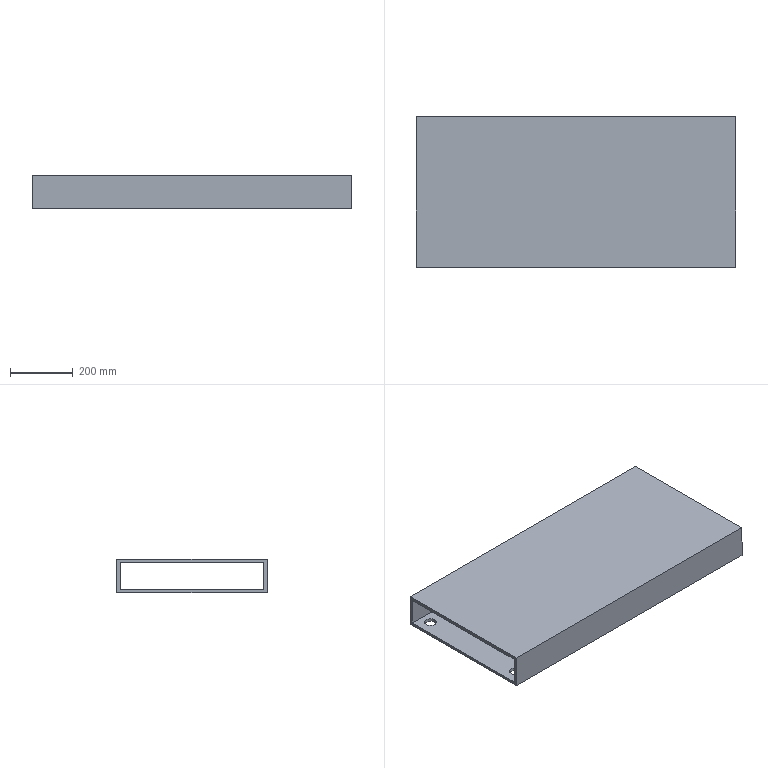Part | SolidWorks | features Cut 1, Extrusion 1, Shell 1 | 1 solid | 18 faces | box 1020 x 480 x 108 mm | volume 11543021 mm3 | plane 10 | cylinder 8 | commonest cylinder face diameters 37.5 x8
STEP:
#1=CARTESIAN_POINT('',(-446.342,191.837,10.));
#2=VERTEX_POINT('',#1);
#3=CARTESIAN_POINT('',(-483.842,191.837,10.));
#4=VERTEX_POINT('',#3);
#5=CARTESIAN_POINT('',(-465.092,191.837,10.));
#6=DIRECTION('',(0.,0.,-1.));
#7=DIRECTION('',(-1.,0.,0.));
#8=AXIS2_PLACEMENT_3D('',#5,#6,#7);
#9=CIRCLE('',#8,18.75);
#10=EDGE_CURVE('',#2,#4,#9,.T.);
#11=ORIENTED_EDGE('',*,*,#10,.F.);
#12=CARTESIAN_POINT('',(-446.342,191.837,0.));
#13=VERTEX_POINT('',#12);
#14=CARTESIAN_POINT('',(-446.342,191.837,10.));
#15=DIRECTION('',(0.,0.,-1.));
#16=VECTOR('',#15,1000.);
#17=LINE('',#14,#16);
#18=EDGE_CURVE('',#2,#13,#17,.T.);
#19=ORIENTED_EDGE('',*,*,#18,.T.);
#20=CARTESIAN_POINT('',(-483.842,191.837,0.));
#21=VERTEX_POINT('',#20);
#22=CARTESIAN_POINT('',(-465.092,191.837,0.));
#23=DIRECTION('',(0.,0.,-1.));
#24=DIRECTION('',(-1.,0.,0.));
#25=AXIS2_PLACEMENT_3D('',#22,#23,#24);
#26=CIRCLE('',#25,18.75);
#27=EDGE_CURVE('',#13,#21,#26,.T.);
#28=ORIENTED_EDGE('',*,*,#27,.T.);
#29=CARTESIAN_POINT('',(-483.842,191.837,10.));
#30=DIRECTION('',(0.,0.,-1.));
#31=VECTOR('',#30,1000.);
#32=LINE('',#29,#31);
#33=EDGE_CURVE('',#4,#21,#32,.T.);
#34=ORIENTED_EDGE('',*,*,#33,.F.);
#35=EDGE_LOOP('',(#11,#19,#28,#34));
#36=FACE_OUTER_BOUND('',#35,.T.);
#37=CARTESIAN_POINT('',(-465.092,191.837,10.));
#38=DIRECTION('',(0.,0.,-1.));
#39=DIRECTION('',(-1.,0.,0.));
#40=AXIS2_PLACEMENT_3D('',#37,#38,#39);
#41=CYLINDRICAL_SURFACE('',#40,18.75);
#42=ADVANCED_FACE('',(#36),#41,.F.);
#43=CARTESIAN_POINT('',(-446.342,-191.837,10.));
#44=VERTEX_POINT('',#43);
#45=CARTESIAN_POINT('',(-483.842,-191.837,10.));
#46=VERTEX_POINT('',#45);
#47=CARTESIAN_POINT('',(-465.092,-191.837,10.));
#48=DIRECTION('',(0.,0.,-1.));
#49=DIRECTION('',(-1.,0.,0.));
#50=AXIS2_PLACEMENT_3D('',#47,#48,#49);
#51=CIRCLE('',#50,18.75);
#52=EDGE_CURVE('',#44,#46,#51,.T.);
#53=ORIENTED_EDGE('',*,*,#52,.F.);
#54=CARTESIAN_POINT('',(-446.342,-191.837,0.));
#55=VERTEX_POINT('',#54);
#56=CARTESIAN_POINT('',(-446.342,-191.837,10.));
#57=DIRECTION('',(0.,0.,-1.));
#58=VECTOR('',#57,1000.);
#59=LINE('',#56,#58);
#60=EDGE_CURVE('',#44,#55,#59,.T.);
#61=ORIENTED_EDGE('',*,*,#60,.T.);
#62=CARTESIAN_POINT('',(-483.842,-191.837,0.));
#63=VERTEX_POINT('',#62);
#64=CARTESIAN_POINT('',(-465.092,-191.837,0.));
#65=DIRECTION('',(0.,0.,-1.));
#66=DIRECTION('',(-1.,0.,0.));
#67=AXIS2_PLACEMENT_3D('',#64,#65,#66);
#68=CIRCLE('',#67,18.75);
#69=EDGE_CURVE('',#55,#63,#68,.T.);
#70=ORIENTED_EDGE('',*,*,#69,.T.);
#71=CARTESIAN_POINT('',(-483.842,-191.837,10.));
#72=DIRECTION('',(0.,0.,-1.));
#73=VECTOR('',#72,1000.);
#74=LINE('',#71,#73);
#75=EDGE_CURVE('',#46,#63,#74,.T.);
#76=ORIENTED_EDGE('',*,*,#75,.F.);
#77=EDGE_LOOP('',(#53,#61,#70,#76));
#78=FACE_OUTER_BOUND('',#77,.T.);
#79=CARTESIAN_POINT('',(-465.092,-191.837,10.));
#80=DIRECTION('',(0.,0.,-1.));
#81=DIRECTION('',(-1.,0.,0.));
#82=AXIS2_PLACEMENT_3D('',#79,#80,#81);
#83=CYLINDRICAL_SURFACE('',#82,18.75);
#84=ADVANCED_FACE('',(#78),#83,.F.);
#85=CARTESIAN_POINT('',(414.283,-192.188,10.));
#86=VERTEX_POINT('',#85);
#87=CARTESIAN_POINT('',(376.783,-192.188,10.));
#88=VERTEX_POINT('',#87);
#89=CARTESIAN_POINT('',(395.533,-192.188,10.));
#90=DIRECTION('',(0.,0.,-1.));
#91=DIRECTION('',(-1.,0.,0.));
#92=AXIS2_PLACEMENT_3D('',#89,#90,#91);
#93=CIRCLE('',#92,18.75);
#94=EDGE_CURVE('',#86,#88,#93,.T.);
#95=ORIENTED_EDGE('',*,*,#94,.F.);
#96=CARTESIAN_POINT('',(414.283,-192.188,0.));
#97=VERTEX_POINT('',#96);
#98=CARTESIAN_POINT('',(414.283,-192.188,10.));
#99=DIRECTION('',(0.,0.,-1.));
#100=VECTOR('',#99,1000.);
#101=LINE('',#98,#100);
#102=EDGE_CURVE('',#86,#97,#101,.T.);
#103=ORIENTED_EDGE('',*,*,#102,.T.);
#104=CARTESIAN_POINT('',(376.783,-192.188,0.));
#105=VERTEX_POINT('',#104);
#106=CARTESIAN_POINT('',(395.533,-192.188,0.));
#107=DIRECTION('',(0.,0.,-1.));
#108=DIRECTION('',(-1.,0.,0.));
#109=AXIS2_PLACEMENT_3D('',#106,#107,#108);
#110=CIRCLE('',#109,18.75);
#111=EDGE_CURVE('',#97,#105,#110,.T.);
#112=ORIENTED_EDGE('',*,*,#111,.T.);
#113=CARTESIAN_POINT('',(376.783,-192.188,10.));
#114=DIRECTION('',(0.,0.,-1.));
#115=VECTOR('',#114,1000.);
#116=LINE('',#113,#115);
#117=EDGE_CURVE('',#88,#105,#116,.T.);
#118=ORIENTED_EDGE('',*,*,#117,.F.);
#119=EDGE_LOOP('',(#95,#103,#112,#118));
#120=FACE_OUTER_BOUND('',#119,.T.);
#121=CARTESIAN_POINT('',(395.533,-192.188,10.));
#122=DIRECTION('',(0.,0.,-1.));
#123=DIRECTION('',(-1.,0.,0.));
#124=AXIS2_PLACEMENT_3D('',#121,#122,#123);
#125=CYLINDRICAL_SURFACE('',#124,18.75);
#126=ADVANCED_FACE('',(#120),#125,.F.);
#127=CARTESIAN_POINT('',(416.221,192.187,10.));
#128=VERTEX_POINT('',#127);
#129=CARTESIAN_POINT('',(378.721,192.187,10.));
#130=VERTEX_POINT('',#129);
#131=CARTESIAN_POINT('',(397.471,192.187,10.));
#132=DIRECTION('',(0.,0.,-1.));
#133=DIRECTION('',(-1.,0.,0.));
#134=AXIS2_PLACEMENT_3D('',#131,#132,#133);
#135=CIRCLE('',#134,18.75);
#136=EDGE_CURVE('',#128,#130,#135,.T.);
#137=ORIENTED_EDGE('',*,*,#136,.F.);
#138=CARTESIAN_POINT('',(416.221,192.187,0.));
#139=VERTEX_POINT('',#138);
#140=CARTESIAN_POINT('',(416.221,192.187,10.));
#141=DIRECTION('',(0.,0.,-1.));
#142=VECTOR('',#141,1000.);
#143=LINE('',#140,#142);
#144=EDGE_CURVE('',#128,#139,#143,.T.);
#145=ORIENTED_EDGE('',*,*,#144,.T.);
#146=CARTESIAN_POINT('',(378.721,192.187,0.));
#147=VERTEX_POINT('',#146);
#148=CARTESIAN_POINT('',(397.471,192.187,0.));
#149=DIRECTION('',(0.,0.,-1.));
#150=DIRECTION('',(-1.,0.,0.));
#151=AXIS2_PLACEMENT_3D('',#148,#149,#150);
#152=CIRCLE('',#151,18.75);
#153=EDGE_CURVE('',#139,#147,#152,.T.);
#154=ORIENTED_EDGE('',*,*,#153,.T.);
#155=CARTESIAN_POINT('',(378.721,192.187,10.));
#156=DIRECTION('',(0.,0.,-1.));
#157=VECTOR('',#156,1000.);
#158=LINE('',#155,#157);
#159=EDGE_CURVE('',#130,#147,#158,.T.);
#160=ORIENTED_EDGE('',*,*,#159,.F.);
#161=EDGE_LOOP('',(#137,#145,#154,#160));
#162=FACE_OUTER_BOUND('',#161,.T.);
#163=CARTESIAN_POINT('',(397.471,192.187,10.));
#164=DIRECTION('',(0.,0.,-1.));
#165=DIRECTION('',(-1.,0.,0.));
#166=AXIS2_PLACEMENT_3D('',#163,#164,#165);
#167=CYLINDRICAL_SURFACE('',#166,18.75);
#168=ADVANCED_FACE('',(#162),#167,.F.);
#169=CARTESIAN_POINT('',(510.,-240.,0.));
#170=VERTEX_POINT('',#169);
#171=CARTESIAN_POINT('',(510.,240.,0.));
#172=VERTEX_POINT('',#171);
#173=CARTESIAN_POINT('',(510.,240.,0.));
#174=DIRECTION('',(0.,1.,0.));
#175=VECTOR('',#174,1000.);
#176=LINE('',#173,#175);
#177=EDGE_CURVE('',#170,#172,#176,.T.);
#178=ORIENTED_EDGE('',*,*,#177,.T.);
#179=CARTESIAN_POINT('',(510.,240.,108.));
#180=VERTEX_POINT('',#179);
#181=CARTESIAN_POINT('',(510.,240.,108.));
#182=DIRECTION('',(0.,0.,-1.));
#183=VECTOR('',#182,1000.);
#184=LINE('',#181,#183);
#185=EDGE_CURVE('',#180,#172,#184,.T.);
#186=ORIENTED_EDGE('',*,*,#185,.F.);
#187=CARTESIAN_POINT('',(510.,-240.,108.));
#188=VERTEX_POINT('',#187);
#189=CARTESIAN_POINT('',(510.,240.,108.));
#190=DIRECTION('',(0.,1.,0.));
#191=VECTOR('',#190,1000.);
#192=LINE('',#189,#191);
#193=EDGE_CURVE('',#188,#180,#192,.T.);
#194=ORIENTED_EDGE('',*,*,#193,.F.);
#195=CARTESIAN_POINT('',(510.,-240.,108.));
#196=DIRECTION('',(0.,0.,-1.));
#197=VECTOR('',#196,1000.);
#198=LINE('',#195,#197);
#199=EDGE_CURVE('',#188,#170,#198,.T.);
#200=ORIENTED_EDGE('',*,*,#199,.T.);
#201=EDGE_LOOP('',(#178,#186,#194,#200));
#202=FACE_OUTER_BOUND('',#201,.T.);
#203=CARTESIAN_POINT('',(510.,-230.,10.));
#204=VERTEX_POINT('',#203);
#205=CARTESIAN_POINT('',(510.,230.,10.));
#206=VERTEX_POINT('',#205);
#207=CARTESIAN_POINT('',(510.,240.,10.));
#208=DIRECTION('',(0.,1.,0.));
#209=VECTOR('',#208,1000.);
#210=LINE('',#207,#209);
#211=EDGE_CURVE('',#204,#206,#210,.T.);
#212=ORIENTED_EDGE('',*,*,#211,.F.);
#213=CARTESIAN_POINT('',(510.,-230.,98.));
#214=VERTEX_POINT('',#213);
#215=CARTESIAN_POINT('',(510.,-230.,108.));
#216=DIRECTION('',(0.,0.,-1.));
#217=VECTOR('',#216,1000.);
#218=LINE('',#215,#217);
#219=EDGE_CURVE('',#214,#204,#218,.T.);
#220=ORIENTED_EDGE('',*,*,#219,.F.);
#221=CARTESIAN_POINT('',(510.,230.,98.));
#222=VERTEX_POINT('',#221);
#223=CARTESIAN_POINT('',(510.,240.,98.));
#224=DIRECTION('',(0.,1.,0.));
#225=VECTOR('',#224,1000.);
#226=LINE('',#223,#225);
#227=EDGE_CURVE('',#214,#222,#226,.T.);
#228=ORIENTED_EDGE('',*,*,#227,.T.);
#229=CARTESIAN_POINT('',(510.,230.,108.));
#230=DIRECTION('',(0.,0.,-1.));
#231=VECTOR('',#230,1000.);
#232=LINE('',#229,#231);
#233=EDGE_CURVE('',#222,#206,#232,.T.);
#234=ORIENTED_EDGE('',*,*,#233,.T.);
#235=EDGE_LOOP('',(#212,#220,#228,#234));
#236=FACE_BOUND('',#235,.T.);
#237=CARTESIAN_POINT('',(510.,240.,108.));
#238=DIRECTION('',(-1.,0.,0.));
#239=DIRECTION('',(0.,-1.,0.));
#240=AXIS2_PLACEMENT_3D('',#237,#238,#239);
#241=PLANE('',#240);
#242=ADVANCED_FACE('',(#202,#236),#241,.F.);
#243=CARTESIAN_POINT('',(-510.,240.,0.));
#244=VERTEX_POINT('',#243);
#245=CARTESIAN_POINT('',(-510.,-240.,0.));
#246=VERTEX_POINT('',#245);
#247=CARTESIAN_POINT('',(-510.,240.,0.));
#248=DIRECTION('',(0.,-1.,0.));
#249=VECTOR('',#248,1000.);
#250=LINE('',#247,#249);
#251=EDGE_CURVE('',#244,#246,#250,.T.);
#252=ORIENTED_EDGE('',*,*,#251,.T.);
#253=CARTESIAN_POINT('',(-510.,-240.,108.));
#254=VERTEX_POINT('',#253);
#255=CARTESIAN_POINT('',(-510.,-240.,108.));
#256=DIRECTION('',(0.,0.,-1.));
#257=VECTOR('',#256,1000.);
#258=LINE('',#255,#257);
#259=EDGE_CURVE('',#254,#246,#258,.T.);
#260=ORIENTED_EDGE('',*,*,#259,.F.);
#261=CARTESIAN_POINT('',(-510.,240.,108.));
#262=VERTEX_POINT('',#261);
#263=CARTESIAN_POINT('',(-510.,240.,108.));
#264=DIRECTION('',(0.,-1.,0.));
#265=VECTOR('',#264,1000.);
#266=LINE('',#263,#265);
#267=EDGE_CURVE('',#262,#254,#266,.T.);
#268=ORIENTED_EDGE('',*,*,#267,.F.);
#269=CARTESIAN_POINT('',(-510.,240.,108.));
#270=DIRECTION('',(0.,0.,-1.));
#271=VECTOR('',#270,1000.);
#272=LINE('',#269,#271);
#273=EDGE_CURVE('',#262,#244,#272,.T.);
#274=ORIENTED_EDGE('',*,*,#273,.T.);
#275=EDGE_LOOP('',(#252,#260,#268,#274));
#276=FACE_OUTER_BOUND('',#275,.T.);
#277=CARTESIAN_POINT('',(-510.,230.,10.));
#278=VERTEX_POINT('',#277);
#279=CARTESIAN_POINT('',(-510.,-230.,10.));
#280=VERTEX_POINT('',#279);
#281=CARTESIAN_POINT('',(-510.,240.,10.));
#282=DIRECTION('',(0.,-1.,0.));
#283=VECTOR('',#282,1000.);
#284=LINE('',#281,#283);
#285=EDGE_CURVE('',#278,#280,#284,.T.);
#286=ORIENTED_EDGE('',*,*,#285,.F.);
#287=CARTESIAN_POINT('',(-510.,230.,98.));
#288=VERTEX_POINT('',#287);
#289=CARTESIAN_POINT('',(-510.,230.,108.));
#290=DIRECTION('',(0.,0.,-1.));
#291=VECTOR('',#290,1000.);
#292=LINE('',#289,#291);
#293=EDGE_CURVE('',#288,#278,#292,.T.);
#294=ORIENTED_EDGE('',*,*,#293,.F.);
#295=CARTESIAN_POINT('',(-510.,-230.,98.));
#296=VERTEX_POINT('',#295);
#297=CARTESIAN_POINT('',(-510.,240.,98.));
#298=DIRECTION('',(0.,-1.,0.));
#299=VECTOR('',#298,1000.);
#300=LINE('',#297,#299);
#301=EDGE_CURVE('',#288,#296,#300,.T.);
#302=ORIENTED_EDGE('',*,*,#301,.T.);
#303=CARTESIAN_POINT('',(-510.,-230.,108.));
#304=DIRECTION('',(0.,0.,-1.));
#305=VECTOR('',#304,1000.);
#306=LINE('',#303,#305);
#307=EDGE_CURVE('',#296,#280,#306,.T.);
#308=ORIENTED_EDGE('',*,*,#307,.T.);
#309=EDGE_LOOP('',(#286,#294,#302,#308));
#310=FACE_BOUND('',#309,.T.);
#311=CARTESIAN_POINT('',(-510.,240.,108.));
#312=DIRECTION('',(1.,0.,0.));
#313=DIRECTION('',(0.,1.,0.));
#314=AXIS2_PLACEMENT_3D('',#311,#312,#313);
#315=PLANE('',#314);
#316=ADVANCED_FACE('',(#276,#310),#315,.F.);
#317=CARTESIAN_POINT('',(-510.,240.,0.));
#318=DIRECTION('',(-1.,0.,0.));
#319=VECTOR('',#318,1000.);
#320=LINE('',#317,#319);
#321=EDGE_CURVE('',#172,#244,#320,.T.);
#322=ORIENTED_EDGE('',*,*,#321,.T.);
#323=ORIENTED_EDGE('',*,*,#273,.F.);
#324=CARTESIAN_POINT('',(-510.,240.,108.));
#325=DIRECTION('',(-1.,0.,0.));
#326=VECTOR('',#325,1000.);
#327=LINE('',#324,#326);
#328=EDGE_CURVE('',#180,#262,#327,.T.);
#329=ORIENTED_EDGE('',*,*,#328,.F.);
#330=ORIENTED_EDGE('',*,*,#185,.T.);
#331=EDGE_LOOP('',(#322,#323,#329,#330));
#332=FACE_OUTER_BOUND('',#331,.T.);
#333=CARTESIAN_POINT('',(-510.,240.,108.));
#334=DIRECTION('',(0.,-1.,0.));
#335=DIRECTION('',(0.,0.,-1.));
#336=AXIS2_PLACEMENT_3D('',#333,#334,#335);
#337=PLANE('',#336);
#338=ADVANCED_FACE('',(#332),#337,.F.);
#339=CARTESIAN_POINT('',(-510.,-240.,0.));
#340=DIRECTION('',(1.,0.,0.));
#341=VECTOR('',#340,1000.);
#342=LINE('',#339,#341);
#343=EDGE_CURVE('',#246,#170,#342,.T.);
#344=ORIENTED_EDGE('',*,*,#343,.T.);
#345=ORIENTED_EDGE('',*,*,#199,.F.);
#346=CARTESIAN_POINT('',(-510.,-240.,108.));
#347=DIRECTION('',(1.,0.,0.));
#348=VECTOR('',#347,1000.);
#349=LINE('',#346,#348);
#350=EDGE_CURVE('',#254,#188,#349,.T.);
#351=ORIENTED_EDGE('',*,*,#350,.F.);
#352=ORIENTED_EDGE('',*,*,#259,.T.);
#353=EDGE_LOOP('',(#344,#345,#351,#352));
#354=FACE_OUTER_BOUND('',#353,.T.);
#355=CARTESIAN_POINT('',(-510.,-240.,108.));
#356=DIRECTION('',(0.,1.,0.));
#357=DIRECTION('',(0.,0.,1.));
#358=AXIS2_PLACEMENT_3D('',#355,#356,#357);
#359=PLANE('',#358);
#360=ADVANCED_FACE('',(#354),#359,.F.);
#361=ORIENTED_EDGE('',*,*,#193,.T.);
#362=ORIENTED_EDGE('',*,*,#328,.T.);
#363=ORIENTED_EDGE('',*,*,#267,.T.);
#364=ORIENTED_EDGE('',*,*,#350,.T.);
#365=EDGE_LOOP('',(#361,#362,#363,#364));
#366=FACE_OUTER_BOUND('',#365,.T.);
#367=CARTESIAN_POINT('',(0.,0.,108.));
#368=DIRECTION('',(0.,0.,1.));
#369=DIRECTION('',(1.,0.,0.));
#370=AXIS2_PLACEMENT_3D('',#367,#368,#369);
#371=PLANE('',#370);
#372=ADVANCED_FACE('',(#366),#371,.T.);
#373=CARTESIAN_POINT('',(-465.092,191.837,0.));
#374=DIRECTION('',(0.,0.,-1.));
#375=DIRECTION('',(-1.,0.,0.));
#376=AXIS2_PLACEMENT_3D('',#373,#374,#375);
#377=CIRCLE('',#376,18.75);
#378=EDGE_CURVE('',#21,#13,#377,.T.);
#379=ORIENTED_EDGE('',*,*,#378,.F.);
#380=ORIENTED_EDGE('',*,*,#27,.F.);
#381=EDGE_LOOP('',(#379,#380));
#382=FACE_BOUND('',#381,.T.);
#383=CARTESIAN_POINT('',(-465.092,-191.837,0.));
#384=DIRECTION('',(0.,0.,-1.));
#385=DIRECTION('',(-1.,0.,0.));
#386=AXIS2_PLACEMENT_3D('',#383,#384,#385);
#387=CIRCLE('',#386,18.75);
#388=EDGE_CURVE('',#63,#55,#387,.T.);
#389=ORIENTED_EDGE('',*,*,#388,.F.);
#390=ORIENTED_EDGE('',*,*,#69,.F.);
#391=EDGE_LOOP('',(#389,#390));
#392=FACE_BOUND('',#391,.T.);
#393=CARTESIAN_POINT('',(395.533,-192.188,0.));
#394=DIRECTION('',(0.,0.,-1.));
#395=DIRECTION('',(-1.,0.,0.));
#396=AXIS2_PLACEMENT_3D('',#393,#394,#395);
#397=CIRCLE('',#396,18.75);
#398=EDGE_CURVE('',#105,#97,#397,.T.);
#399=ORIENTED_EDGE('',*,*,#398,.F.);
#400=ORIENTED_EDGE('',*,*,#111,.F.);
#401=EDGE_LOOP('',(#399,#400));
#402=FACE_BOUND('',#401,.T.);
#403=CARTESIAN_POINT('',(397.471,192.187,0.));
#404=DIRECTION('',(0.,0.,-1.));
#405=DIRECTION('',(-1.,0.,0.));
#406=AXIS2_PLACEMENT_3D('',#403,#404,#405);
#407=CIRCLE('',#406,18.75);
#408=EDGE_CURVE('',#147,#139,#407,.T.);
#409=ORIENTED_EDGE('',*,*,#408,.F.);
#410=ORIENTED_EDGE('',*,*,#153,.F.);
#411=EDGE_LOOP('',(#409,#410));
#412=FACE_BOUND('',#411,.T.);
#413=ORIENTED_EDGE('',*,*,#177,.F.);
#414=ORIENTED_EDGE('',*,*,#343,.F.);
#415=ORIENTED_EDGE('',*,*,#251,.F.);
#416=ORIENTED_EDGE('',*,*,#321,.F.);
#417=EDGE_LOOP('',(#413,#414,#415,#416));
#418=FACE_OUTER_BOUND('',#417,.T.);
#419=CARTESIAN_POINT('',(0.,0.,0.));
#420=DIRECTION('',(0.,0.,1.));
#421=DIRECTION('',(1.,0.,0.));
#422=AXIS2_PLACEMENT_3D('',#419,#420,#421);
#423=PLANE('',#422);
#424=ADVANCED_FACE('',(#382,#392,#402,#412,#418),#423,.F.);
#425=CARTESIAN_POINT('',(-510.,230.,10.));
#426=DIRECTION('',(-1.,0.,0.));
#427=VECTOR('',#426,1000.);
#428=LINE('',#425,#427);
#429=EDGE_CURVE('',#206,#278,#428,.T.);
#430=ORIENTED_EDGE('',*,*,#429,.F.);
#431=ORIENTED_EDGE('',*,*,#233,.F.);
#432=CARTESIAN_POINT('',(-510.,230.,98.));
#433=DIRECTION('',(-1.,0.,0.));
#434=VECTOR('',#433,1000.);
#435=LINE('',#432,#434);
#436=EDGE_CURVE('',#222,#288,#435,.T.);
#437=ORIENTED_EDGE('',*,*,#436,.T.);
#438=ORIENTED_EDGE('',*,*,#293,.T.);
#439=EDGE_LOOP('',(#430,#431,#437,#438));
#440=FACE_OUTER_BOUND('',#439,.T.);
#441=CARTESIAN_POINT('',(-510.,230.,108.));
#442=DIRECTION('',(0.,-1.,0.));
#443=DIRECTION('',(0.,0.,-1.));
#444=AXIS2_PLACEMENT_3D('',#441,#442,#443);
#445=PLANE('',#444);
#446=ADVANCED_FACE('',(#440),#445,.T.);
#447=CARTESIAN_POINT('',(-510.,-230.,10.));
#448=DIRECTION('',(1.,0.,0.));
#449=VECTOR('',#448,1000.);
#450=LINE('',#447,#449);
#451=EDGE_CURVE('',#280,#204,#450,.T.);
#452=ORIENTED_EDGE('',*,*,#451,.F.);
#453=ORIENTED_EDGE('',*,*,#307,.F.);
#454=CARTESIAN_POINT('',(-510.,-230.,98.));
#455=DIRECTION('',(1.,0.,0.));
#456=VECTOR('',#455,1000.);
#457=LINE('',#454,#456);
#458=EDGE_CURVE('',#296,#214,#457,.T.);
#459=ORIENTED_EDGE('',*,*,#458,.T.);
#460=ORIENTED_EDGE('',*,*,#219,.T.);
#461=EDGE_LOOP('',(#452,#453,#459,#460));
#462=FACE_OUTER_BOUND('',#461,.T.);
#463=CARTESIAN_POINT('',(-510.,-230.,108.));
#464=DIRECTION('',(0.,1.,0.));
#465=DIRECTION('',(0.,0.,1.));
#466=AXIS2_PLACEMENT_3D('',#463,#464,#465);
#467=PLANE('',#466);
#468=ADVANCED_FACE('',(#462),#467,.T.);
#469=ORIENTED_EDGE('',*,*,#227,.F.);
#470=ORIENTED_EDGE('',*,*,#458,.F.);
#471=ORIENTED_EDGE('',*,*,#301,.F.);
#472=ORIENTED_EDGE('',*,*,#436,.F.);
#473=EDGE_LOOP('',(#469,#470,#471,#472));
#474=FACE_OUTER_BOUND('',#473,.T.);
#475=CARTESIAN_POINT('',(0.,0.,98.));
#476=DIRECTION('',(0.,0.,1.));
#477=DIRECTION('',(1.,0.,0.));
#478=AXIS2_PLACEMENT_3D('',#475,#476,#477);
#479=PLANE('',#478);
#480=ADVANCED_FACE('',(#474),#479,.F.);
#481=CARTESIAN_POINT('',(-465.092,191.837,10.));
#482=DIRECTION('',(0.,0.,-1.));
#483=DIRECTION('',(-1.,0.,0.));
#484=AXIS2_PLACEMENT_3D('',#481,#482,#483);
#485=CIRCLE('',#484,18.75);
#486=EDGE_CURVE('',#4,#2,#485,.T.);
#487=ORIENTED_EDGE('',*,*,#486,.T.);
#488=ORIENTED_EDGE('',*,*,#10,.T.);
#489=EDGE_LOOP('',(#487,#488));
#490=FACE_BOUND('',#489,.T.);
#491=CARTESIAN_POINT('',(-465.092,-191.837,10.));
#492=DIRECTION('',(0.,0.,-1.));
#493=DIRECTION('',(-1.,0.,0.));
#494=AXIS2_PLACEMENT_3D('',#491,#492,#493);
#495=CIRCLE('',#494,18.75);
#496=EDGE_CURVE('',#46,#44,#495,.T.);
#497=ORIENTED_EDGE('',*,*,#496,.T.);
#498=ORIENTED_EDGE('',*,*,#52,.T.);
#499=EDGE_LOOP('',(#497,#498));
#500=FACE_BOUND('',#499,.T.);
#501=CARTESIAN_POINT('',(395.533,-192.188,10.));
#502=DIRECTION('',(0.,0.,-1.));
#503=DIRECTION('',(-1.,0.,0.));
#504=AXIS2_PLACEMENT_3D('',#501,#502,#503);
#505=CIRCLE('',#504,18.75);
#506=EDGE_CURVE('',#88,#86,#505,.T.);
#507=ORIENTED_EDGE('',*,*,#506,.T.);
#508=ORIENTED_EDGE('',*,*,#94,.T.);
#509=EDGE_LOOP('',(#507,#508));
#510=FACE_BOUND('',#509,.T.);
#511=CARTESIAN_POINT('',(397.471,192.187,10.));
#512=DIRECTION('',(0.,0.,-1.));
#513=DIRECTION('',(-1.,0.,0.));
#514=AXIS2_PLACEMENT_3D('',#511,#512,#513);
#515=CIRCLE('',#514,18.75);
#516=EDGE_CURVE('',#130,#128,#515,.T.);
#517=ORIENTED_EDGE('',*,*,#516,.T.);
#518=ORIENTED_EDGE('',*,*,#136,.T.);
#519=EDGE_LOOP('',(#517,#518));
#520=FACE_BOUND('',#519,.T.);
#521=ORIENTED_EDGE('',*,*,#211,.T.);
#522=ORIENTED_EDGE('',*,*,#429,.T.);
#523=ORIENTED_EDGE('',*,*,#285,.T.);
#524=ORIENTED_EDGE('',*,*,#451,.T.);
#525=EDGE_LOOP('',(#521,#522,#523,#524));
#526=FACE_OUTER_BOUND('',#525,.T.);
#527=CARTESIAN_POINT('',(0.,0.,10.));
#528=DIRECTION('',(0.,0.,1.));
#529=DIRECTION('',(1.,0.,0.));
#530=AXIS2_PLACEMENT_3D('',#527,#528,#529);
#531=PLANE('',#530);
#532=ADVANCED_FACE('',(#490,#500,#510,#520,#526),#531,.T.);
#533=ORIENTED_EDGE('',*,*,#144,.F.);
#534=ORIENTED_EDGE('',*,*,#516,.F.);
#535=ORIENTED_EDGE('',*,*,#159,.T.);
#536=ORIENTED_EDGE('',*,*,#408,.T.);
#537=EDGE_LOOP('',(#533,#534,#535,#536));
#538=FACE_OUTER_BOUND('',#537,.T.);
#539=CARTESIAN_POINT('',(397.471,192.187,10.));
#540=DIRECTION('',(0.,0.,-1.));
#541=DIRECTION('',(-1.,0.,0.));
#542=AXIS2_PLACEMENT_3D('',#539,#540,#541);
#543=CYLINDRICAL_SURFACE('',#542,18.75);
#544=ADVANCED_FACE('',(#538),#543,.F.);
#545=ORIENTED_EDGE('',*,*,#102,.F.);
#546=ORIENTED_EDGE('',*,*,#506,.F.);
#547=ORIENTED_EDGE('',*,*,#117,.T.);
#548=ORIENTED_EDGE('',*,*,#398,.T.);
#549=EDGE_LOOP('',(#545,#546,#547,#548));
#550=FACE_OUTER_BOUND('',#549,.T.);
#551=CARTESIAN_POINT('',(395.533,-192.188,10.));
#552=DIRECTION('',(0.,0.,-1.));
#553=DIRECTION('',(-1.,0.,0.));
#554=AXIS2_PLACEMENT_3D('',#551,#552,#553);
#555=CYLINDRICAL_SURFACE('',#554,18.75);
#556=ADVANCED_FACE('',(#550),#555,.F.);
#557=ORIENTED_EDGE('',*,*,#60,.F.);
#558=ORIENTED_EDGE('',*,*,#496,.F.);
#559=ORIENTED_EDGE('',*,*,#75,.T.);
#560=ORIENTED_EDGE('',*,*,#388,.T.);
#561=EDGE_LOOP('',(#557,#558,#559,#560));
#562=FACE_OUTER_BOUND('',#561,.T.);
#563=CARTESIAN_POINT('',(-465.092,-191.837,10.));
#564=DIRECTION('',(0.,0.,-1.));
#565=DIRECTION('',(-1.,0.,0.));
#566=AXIS2_PLACEMENT_3D('',#563,#564,#565);
#567=CYLINDRICAL_SURFACE('',#566,18.75);
#568=ADVANCED_FACE('',(#562),#567,.F.);
#569=ORIENTED_EDGE('',*,*,#18,.F.);
#570=ORIENTED_EDGE('',*,*,#486,.F.);
#571=ORIENTED_EDGE('',*,*,#33,.T.);
#572=ORIENTED_EDGE('',*,*,#378,.T.);
#573=EDGE_LOOP('',(#569,#570,#571,#572));
#574=FACE_OUTER_BOUND('',#573,.T.);
#575=CARTESIAN_POINT('',(-465.092,191.837,10.));
#576=DIRECTION('',(0.,0.,-1.));
#577=DIRECTION('',(-1.,0.,0.));
#578=AXIS2_PLACEMENT_3D('',#575,#576,#577);
#579=CYLINDRICAL_SURFACE('',#578,18.75);
#580=ADVANCED_FACE('',(#574),#579,.F.);
#581=CLOSED_SHELL('',(#42,#84,#126,#168,#242,#316,#338,#360,#372,#424,#446,#468,#480,#532,#544,#556,#568,#580));
#582=MANIFOLD_SOLID_BREP('',#581);
#583=CARTESIAN_POINT('',(0.,0.,0.));
#584=DIRECTION('',(0.,0.,1.));
#585=DIRECTION('',(1.,0.,0.));
#586=AXIS2_PLACEMENT_3D('',#583,#584,#585);
#587=(LENGTH_UNIT()NAMED_UNIT(*)SI_UNIT(.MILLI.,.METRE.));
#588=UNCERTAINTY_MEASURE_WITH_UNIT(LENGTH_MEASURE(0.00001),#587,'','');
#589=(NAMED_UNIT(*)PLANE_ANGLE_UNIT()SI_UNIT($,.RADIAN.));
#590=(NAMED_UNIT(*)SI_UNIT($,.STERADIAN.)SOLID_ANGLE_UNIT());
#591=(GEOMETRIC_REPRESENTATION_CONTEXT(3)GLOBAL_UNCERTAINTY_ASSIGNED_CONTEXT((#588))GLOBAL_UNIT_ASSIGNED_CONTEXT((#587,#589,#590))REPRESENTATION_CONTEXT('',''));
#592=ADVANCED_BREP_SHAPE_REPRESENTATION('',(#582,#586),#591);